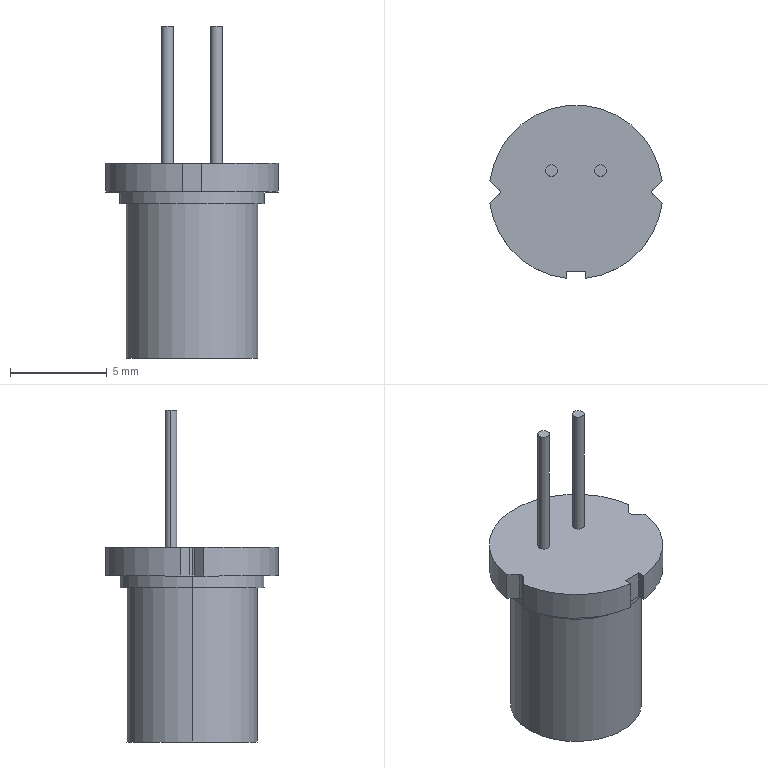Part | SolidWorks | features ICE 5, Dome 1, Extrusion 1, Fillet 1, MoveFace 1 | 1 solid | 31 faces | box 8.917 x 8.972 x 17.2 mm | volume 386.528 mm3 | cylinder 16 | plane 13 | sphere 2 | commonest cylinder face diameters 0.6 x4 0.4 x3 9 x3 5.8 x2 6.8 x2 7.5 x2
STEP:
#1=CARTESIAN_POINT('',(0.,0.,0.1));
#2=VERTEX_POINT('',#1);
#3=CARTESIAN_POINT('',(2.9,0.,3.));
#4=VERTEX_POINT('',#3);
#5=CARTESIAN_POINT('',(0.,0.,3.));
#6=DIRECTION('',(0.,-1.,0.));
#7=DIRECTION('',(1.,0.,0.));
#8=AXIS2_PLACEMENT_3D('',#5,#6,#7);
#9=CIRCLE('',#8,2.9);
#10=EDGE_CURVE('',#2,#4,#9,.T.);
#11=ORIENTED_EDGE('',*,*,#10,.F.);
#12=CARTESIAN_POINT('',(-2.9,0.,3.));
#13=VERTEX_POINT('',#12);
#14=CARTESIAN_POINT('',(0.,0.,3.));
#15=DIRECTION('',(0.,1.,0.));
#16=DIRECTION('',(-1.,0.,0.));
#17=AXIS2_PLACEMENT_3D('',#14,#15,#16);
#18=CIRCLE('',#17,2.9);
#19=EDGE_CURVE('',#2,#13,#18,.T.);
#20=ORIENTED_EDGE('',*,*,#19,.T.);
#21=CARTESIAN_POINT('',(0.,0.,3.));
#22=DIRECTION('',(0.,0.,-1.));
#23=DIRECTION('',(-1.,0.,0.));
#24=AXIS2_PLACEMENT_3D('',#21,#22,#23);
#25=CIRCLE('',#24,2.9);
#26=EDGE_CURVE('',#13,#4,#25,.T.);
#27=ORIENTED_EDGE('',*,*,#26,.T.);
#28=EDGE_LOOP('',(#11,#20,#27));
#29=FACE_OUTER_BOUND('',#28,.T.);
#30=CARTESIAN_POINT('',(0.,0.,3.));
#31=DIRECTION('',(0.,1.,0.));
#32=DIRECTION('',(1.,0.,0.));
#33=AXIS2_PLACEMENT_3D('',#30,#31,#32);
#34=SPHERICAL_SURFACE('',#33,2.9);
#35=ADVANCED_FACE('',(#29),#34,.T.);
#36=CARTESIAN_POINT('',(0.,0.,3.));
#37=DIRECTION('',(0.,0.,-1.));
#38=DIRECTION('',(-1.,0.,0.));
#39=AXIS2_PLACEMENT_3D('',#36,#37,#38);
#40=CIRCLE('',#39,2.9);
#41=EDGE_CURVE('',#4,#13,#40,.T.);
#42=ORIENTED_EDGE('',*,*,#41,.F.);
#43=CARTESIAN_POINT('',(2.9,0.,0.));
#44=VERTEX_POINT('',#43);
#45=CARTESIAN_POINT('',(2.9,0.,3.));
#46=DIRECTION('',(0.,0.,-1.));
#47=VECTOR('',#46,1000.);
#48=LINE('',#45,#47);
#49=EDGE_CURVE('',#4,#44,#48,.T.);
#50=ORIENTED_EDGE('',*,*,#49,.T.);
#51=CARTESIAN_POINT('',(-2.9,0.,0.));
#52=VERTEX_POINT('',#51);
#53=CARTESIAN_POINT('',(0.,0.,0.));
#54=DIRECTION('',(0.,0.,-1.));
#55=DIRECTION('',(-1.,0.,0.));
#56=AXIS2_PLACEMENT_3D('',#53,#54,#55);
#57=CIRCLE('',#56,2.9);
#58=EDGE_CURVE('',#44,#52,#57,.T.);
#59=ORIENTED_EDGE('',*,*,#58,.T.);
#60=CARTESIAN_POINT('',(-2.9,0.,3.));
#61=DIRECTION('',(0.,0.,-1.));
#62=VECTOR('',#61,1000.);
#63=LINE('',#60,#62);
#64=EDGE_CURVE('',#13,#52,#63,.T.);
#65=ORIENTED_EDGE('',*,*,#64,.F.);
#66=EDGE_LOOP('',(#42,#50,#59,#65));
#67=FACE_OUTER_BOUND('',#66,.T.);
#68=CARTESIAN_POINT('',(0.,0.,3.));
#69=DIRECTION('',(0.,0.,-1.));
#70=DIRECTION('',(-1.,0.,0.));
#71=AXIS2_PLACEMENT_3D('',#68,#69,#70);
#72=CYLINDRICAL_SURFACE('',#71,2.9);
#73=ADVANCED_FACE('',(#67),#72,.F.);
#74=CARTESIAN_POINT('',(3.4,0.,8.));
#75=VERTEX_POINT('',#74);
#76=CARTESIAN_POINT('',(-3.4,0.,8.));
#77=VERTEX_POINT('',#76);
#78=CARTESIAN_POINT('',(0.,0.,8.));
#79=DIRECTION('',(0.,0.,1.));
#80=DIRECTION('',(1.,0.,0.));
#81=AXIS2_PLACEMENT_3D('',#78,#79,#80);
#82=CIRCLE('',#81,3.4);
#83=EDGE_CURVE('',#75,#77,#82,.T.);
#84=ORIENTED_EDGE('',*,*,#83,.F.);
#85=CARTESIAN_POINT('',(3.4,0.,0.));
#86=VERTEX_POINT('',#85);
#87=CARTESIAN_POINT('',(3.4,0.,8.6));
#88=DIRECTION('',(0.,0.,-1.));
#89=VECTOR('',#88,1000.);
#90=LINE('',#87,#89);
#91=EDGE_CURVE('',#75,#86,#90,.T.);
#92=ORIENTED_EDGE('',*,*,#91,.T.);
#93=CARTESIAN_POINT('',(-3.4,0.,0.));
#94=VERTEX_POINT('',#93);
#95=CARTESIAN_POINT('',(0.,0.,0.));
#96=DIRECTION('',(0.,0.,1.));
#97=DIRECTION('',(1.,0.,0.));
#98=AXIS2_PLACEMENT_3D('',#95,#96,#97);
#99=CIRCLE('',#98,3.4);
#100=EDGE_CURVE('',#86,#94,#99,.T.);
#101=ORIENTED_EDGE('',*,*,#100,.T.);
#102=CARTESIAN_POINT('',(-3.4,0.,8.6));
#103=DIRECTION('',(0.,0.,-1.));
#104=VECTOR('',#103,1000.);
#105=LINE('',#102,#104);
#106=EDGE_CURVE('',#77,#94,#105,.T.);
#107=ORIENTED_EDGE('',*,*,#106,.F.);
#108=EDGE_LOOP('',(#84,#92,#101,#107));
#109=FACE_OUTER_BOUND('',#108,.T.);
#110=CARTESIAN_POINT('',(0.,0.,8.6));
#111=DIRECTION('',(0.,0.,-1.));
#112=DIRECTION('',(-1.,0.,0.));
#113=AXIS2_PLACEMENT_3D('',#110,#111,#112);
#114=CYLINDRICAL_SURFACE('',#113,3.4);
#115=ADVANCED_FACE('',(#109),#114,.T.);
#116=CARTESIAN_POINT('',(3.75,0.,8.));
#117=VERTEX_POINT('',#116);
#118=CARTESIAN_POINT('',(-3.75,0.,8.));
#119=VERTEX_POINT('',#118);
#120=CARTESIAN_POINT('',(0.,0.,8.));
#121=DIRECTION('',(0.,0.,1.));
#122=DIRECTION('',(1.,0.,0.));
#123=AXIS2_PLACEMENT_3D('',#120,#121,#122);
#124=CIRCLE('',#123,3.75);
#125=EDGE_CURVE('',#117,#119,#124,.T.);
#126=ORIENTED_EDGE('',*,*,#125,.T.);
#127=CARTESIAN_POINT('',(-3.75,0.,8.6));
#128=VERTEX_POINT('',#127);
#129=CARTESIAN_POINT('',(-3.75,0.,-4.807));
#130=DIRECTION('',(0.,0.,1.));
#131=VECTOR('',#130,1000.);
#132=LINE('',#129,#131);
#133=EDGE_CURVE('',#119,#128,#132,.T.);
#134=ORIENTED_EDGE('',*,*,#133,.T.);
#135=CARTESIAN_POINT('',(3.75,0.,8.6));
#136=VERTEX_POINT('',#135);
#137=CARTESIAN_POINT('',(0.,0.,8.6));
#138=DIRECTION('',(0.,0.,-1.));
#139=DIRECTION('',(1.,0.,0.));
#140=AXIS2_PLACEMENT_3D('',#137,#138,#139);
#141=CIRCLE('',#140,3.75);
#142=EDGE_CURVE('',#128,#136,#141,.T.);
#143=ORIENTED_EDGE('',*,*,#142,.T.);
#144=CARTESIAN_POINT('',(3.75,0.,-4.807));
#145=DIRECTION('',(0.,0.,1.));
#146=VECTOR('',#145,1000.);
#147=LINE('',#144,#146);
#148=EDGE_CURVE('',#117,#136,#147,.T.);
#149=ORIENTED_EDGE('',*,*,#148,.F.);
#150=EDGE_LOOP('',(#126,#134,#143,#149));
#151=FACE_OUTER_BOUND('',#150,.T.);
#152=CARTESIAN_POINT('',(0.,0.,-4.807));
#153=DIRECTION('',(0.,0.,1.));
#154=DIRECTION('',(1.,0.,0.));
#155=AXIS2_PLACEMENT_3D('',#152,#153,#154);
#156=CYLINDRICAL_SURFACE('',#155,3.75);
#157=ADVANCED_FACE('',(#151),#156,.T.);
#158=CARTESIAN_POINT('',(-3.933,0.,8.6));
#159=VERTEX_POINT('',#158);
#160=CARTESIAN_POINT('',(-3.991,0.1414,8.6));
#161=VERTEX_POINT('',#160);
#162=CARTESIAN_POINT('',(-4.133,0.,8.6));
#163=DIRECTION('',(0.,0.,1.));
#164=DIRECTION('',(1.,0.,0.));
#165=AXIS2_PLACEMENT_3D('',#162,#163,#164);
#166=CIRCLE('',#165,0.2);
#167=EDGE_CURVE('',#159,#161,#166,.T.);
#168=ORIENTED_EDGE('',*,*,#167,.F.);
#169=CARTESIAN_POINT('',(-3.933,0.,10.1));
#170=VERTEX_POINT('',#169);
#171=CARTESIAN_POINT('',(-3.933,0.,11.949));
#172=DIRECTION('',(0.,0.,1.));
#173=VECTOR('',#172,1000.);
#174=LINE('',#171,#173);
#175=EDGE_CURVE('',#159,#170,#174,.T.);
#176=ORIENTED_EDGE('',*,*,#175,.T.);
#177=CARTESIAN_POINT('',(-3.991,0.1414,10.1));
#178=VERTEX_POINT('',#177);
#179=CARTESIAN_POINT('',(-4.133,0.,10.1));
#180=DIRECTION('',(0.,0.,-1.));
#181=DIRECTION('',(1.,0.,0.));
#182=AXIS2_PLACEMENT_3D('',#179,#180,#181);
#183=CIRCLE('',#182,0.2);
#184=EDGE_CURVE('',#178,#170,#183,.T.);
#185=ORIENTED_EDGE('',*,*,#184,.F.);
#186=CARTESIAN_POINT('',(-3.991,0.1414,10.2));
#187=DIRECTION('',(0.,0.,1.));
#188=VECTOR('',#187,1000.);
#189=LINE('',#186,#188);
#190=EDGE_CURVE('',#161,#178,#189,.T.);
#191=ORIENTED_EDGE('',*,*,#190,.F.);
#192=EDGE_LOOP('',(#168,#176,#185,#191));
#193=FACE_OUTER_BOUND('',#192,.T.);
#194=CARTESIAN_POINT('',(-4.133,0.,11.949));
#195=DIRECTION('',(0.,0.,1.));
#196=DIRECTION('',(1.,0.,0.));
#197=AXIS2_PLACEMENT_3D('',#194,#195,#196);
#198=CYLINDRICAL_SURFACE('',#197,0.2);
#199=ADVANCED_FACE('',(#193),#198,.F.);
#200=CARTESIAN_POINT('',(1.57,1.1,17.2));
#201=VERTEX_POINT('',#200);
#202=CARTESIAN_POINT('',(0.97,1.1,17.2));
#203=VERTEX_POINT('',#202);
#204=CARTESIAN_POINT('',(1.27,1.1,17.2));
#205=DIRECTION('',(0.,0.,1.));
#206=DIRECTION('',(1.,0.,0.));
#207=AXIS2_PLACEMENT_3D('',#204,#205,#206);
#208=CIRCLE('',#207,0.3);
#209=EDGE_CURVE('',#201,#203,#208,.T.);
#210=ORIENTED_EDGE('',*,*,#209,.F.);
#211=CARTESIAN_POINT('',(1.57,1.1,10.1));
#212=VERTEX_POINT('',#211);
#213=CARTESIAN_POINT('',(1.57,1.1,17.2));
#214=DIRECTION('',(0.,0.,-1.));
#215=VECTOR('',#214,1000.);
#216=LINE('',#213,#215);
#217=EDGE_CURVE('',#201,#212,#216,.T.);
#218=ORIENTED_EDGE('',*,*,#217,.T.);
#219=CARTESIAN_POINT('',(0.97,1.1,10.1));
#220=VERTEX_POINT('',#219);
#221=CARTESIAN_POINT('',(1.27,1.1,10.1));
#222=DIRECTION('',(0.,0.,1.));
#223=DIRECTION('',(1.,0.,0.));
#224=AXIS2_PLACEMENT_3D('',#221,#222,#223);
#225=CIRCLE('',#224,0.3);
#226=EDGE_CURVE('',#212,#220,#225,.T.);
#227=ORIENTED_EDGE('',*,*,#226,.T.);
#228=CARTESIAN_POINT('',(0.97,1.1,17.2));
#229=DIRECTION('',(0.,0.,-1.));
#230=VECTOR('',#229,1000.);
#231=LINE('',#228,#230);
#232=EDGE_CURVE('',#203,#220,#231,.T.);
#233=ORIENTED_EDGE('',*,*,#232,.F.);
#234=EDGE_LOOP('',(#210,#218,#227,#233));
#235=FACE_OUTER_BOUND('',#234,.T.);
#236=CARTESIAN_POINT('',(1.27,1.1,17.2));
#237=DIRECTION('',(0.,0.,-1.));
#238=DIRECTION('',(-1.,0.,0.));
#239=AXIS2_PLACEMENT_3D('',#236,#237,#238);
#240=CYLINDRICAL_SURFACE('',#239,0.3);
#241=ADVANCED_FACE('',(#235),#240,.T.);
#242=CARTESIAN_POINT('',(-0.97,1.1,17.2));
#243=VERTEX_POINT('',#242);
#244=CARTESIAN_POINT('',(-1.57,1.1,17.2));
#245=VERTEX_POINT('',#244);
#246=CARTESIAN_POINT('',(-1.27,1.1,17.2));
#247=DIRECTION('',(0.,0.,1.));
#248=DIRECTION('',(1.,0.,0.));
#249=AXIS2_PLACEMENT_3D('',#246,#247,#248);
#250=CIRCLE('',#249,0.3);
#251=EDGE_CURVE('',#243,#245,#250,.T.);
#252=ORIENTED_EDGE('',*,*,#251,.F.);
#253=CARTESIAN_POINT('',(-0.97,1.1,10.1));
#254=VERTEX_POINT('',#253);
#255=CARTESIAN_POINT('',(-0.97,1.1,17.2));
#256=DIRECTION('',(0.,0.,-1.));
#257=VECTOR('',#256,1000.);
#258=LINE('',#255,#257);
#259=EDGE_CURVE('',#243,#254,#258,.T.);
#260=ORIENTED_EDGE('',*,*,#259,.T.);
#261=CARTESIAN_POINT('',(-1.57,1.1,10.1));
#262=VERTEX_POINT('',#261);
#263=CARTESIAN_POINT('',(-1.27,1.1,10.1));
#264=DIRECTION('',(0.,0.,1.));
#265=DIRECTION('',(1.,0.,0.));
#266=AXIS2_PLACEMENT_3D('',#263,#264,#265);
#267=CIRCLE('',#266,0.3);
#268=EDGE_CURVE('',#254,#262,#267,.T.);
#269=ORIENTED_EDGE('',*,*,#268,.T.);
#270=CARTESIAN_POINT('',(-1.57,1.1,17.2));
#271=DIRECTION('',(0.,0.,-1.));
#272=VECTOR('',#271,1000.);
#273=LINE('',#270,#272);
#274=EDGE_CURVE('',#245,#262,#273,.T.);
#275=ORIENTED_EDGE('',*,*,#274,.F.);
#276=EDGE_LOOP('',(#252,#260,#269,#275));
#277=FACE_OUTER_BOUND('',#276,.T.);
#278=CARTESIAN_POINT('',(-1.27,1.1,17.2));
#279=DIRECTION('',(0.,0.,-1.));
#280=DIRECTION('',(-1.,0.,0.));
#281=AXIS2_PLACEMENT_3D('',#278,#279,#280);
#282=CYLINDRICAL_SURFACE('',#281,0.3);
#283=ADVANCED_FACE('',(#277),#282,.T.);
#284=CARTESIAN_POINT('',(-4.459,-0.6086,8.6));
#285=VERTEX_POINT('',#284);
#286=CARTESIAN_POINT('',(-0.5,-4.472,8.6));
#287=VERTEX_POINT('',#286);
#288=CARTESIAN_POINT('',(0.,0.,8.6));
#289=DIRECTION('',(0.,0.,1.));
#290=DIRECTION('',(1.,0.,0.));
#291=AXIS2_PLACEMENT_3D('',#288,#289,#290);
#292=CIRCLE('',#291,4.5);
#293=EDGE_CURVE('',#285,#287,#292,.T.);
#294=ORIENTED_EDGE('',*,*,#293,.T.);
#295=CARTESIAN_POINT('',(-0.5,-4.472,10.1));
#296=VERTEX_POINT('',#295);
#297=CARTESIAN_POINT('',(-0.5,-4.472,10.2));
#298=DIRECTION('',(0.,0.,1.));
#299=VECTOR('',#298,1000.);
#300=LINE('',#297,#299);
#301=EDGE_CURVE('',#287,#296,#300,.T.);
#302=ORIENTED_EDGE('',*,*,#301,.T.);
#303=CARTESIAN_POINT('',(-4.459,-0.6086,10.1));
#304=VERTEX_POINT('',#303);
#305=CARTESIAN_POINT('',(0.,0.,10.1));
#306=DIRECTION('',(0.,0.,1.));
#307=DIRECTION('',(1.,0.,0.));
#308=AXIS2_PLACEMENT_3D('',#305,#306,#307);
#309=CIRCLE('',#308,4.5);
#310=EDGE_CURVE('',#304,#296,#309,.T.);
#311=ORIENTED_EDGE('',*,*,#310,.F.);
#312=CARTESIAN_POINT('',(-4.459,-0.6086,10.2));
#313=DIRECTION('',(0.,0.,-1.));
#314=VECTOR('',#313,1000.);
#315=LINE('',#312,#314);
#316=EDGE_CURVE('',#304,#285,#315,.T.);
#317=ORIENTED_EDGE('',*,*,#316,.T.);
#318=EDGE_LOOP('',(#294,#302,#311,#317));
#319=FACE_OUTER_BOUND('',#318,.T.);
#320=CARTESIAN_POINT('',(0.,0.,10.2));
#321=DIRECTION('',(0.,0.,-1.));
#322=DIRECTION('',(-1.,0.,0.));
#323=AXIS2_PLACEMENT_3D('',#320,#321,#322);
#324=CYLINDRICAL_SURFACE('',#323,4.5);
#325=ADVANCED_FACE('',(#319),#324,.T.);
#326=CARTESIAN_POINT('',(4.459,0.6086,8.6));
#327=VERTEX_POINT('',#326);
#328=CARTESIAN_POINT('',(-4.459,0.6086,8.6));
#329=VERTEX_POINT('',#328);
#330=CARTESIAN_POINT('',(0.,0.,8.6));
#331=DIRECTION('',(0.,0.,1.));
#332=DIRECTION('',(1.,0.,0.));
#333=AXIS2_PLACEMENT_3D('',#330,#331,#332);
#334=CIRCLE('',#333,4.5);
#335=EDGE_CURVE('',#327,#329,#334,.T.);
#336=ORIENTED_EDGE('',*,*,#335,.T.);
#337=CARTESIAN_POINT('',(-4.459,0.6086,10.1));
#338=VERTEX_POINT('',#337);
#339=CARTESIAN_POINT('',(-4.459,0.6086,10.2));
#340=DIRECTION('',(0.,0.,1.));
#341=VECTOR('',#340,1000.);
#342=LINE('',#339,#341);
#343=EDGE_CURVE('',#329,#338,#342,.T.);
#344=ORIENTED_EDGE('',*,*,#343,.T.);
#345=CARTESIAN_POINT('',(4.459,0.6086,10.1));
#346=VERTEX_POINT('',#345);
#347=CARTESIAN_POINT('',(0.,0.,10.1));
#348=DIRECTION('',(0.,0.,1.));
#349=DIRECTION('',(1.,0.,0.));
#350=AXIS2_PLACEMENT_3D('',#347,#348,#349);
#351=CIRCLE('',#350,4.5);
#352=EDGE_CURVE('',#346,#338,#351,.T.);
#353=ORIENTED_EDGE('',*,*,#352,.F.);
#354=CARTESIAN_POINT('',(4.459,0.6086,10.2));
#355=DIRECTION('',(0.,0.,-1.));
#356=VECTOR('',#355,1000.);
#357=LINE('',#354,#356);
#358=EDGE_CURVE('',#346,#327,#357,.T.);
#359=ORIENTED_EDGE('',*,*,#358,.T.);
#360=EDGE_LOOP('',(#336,#344,#353,#359));
#361=FACE_OUTER_BOUND('',#360,.T.);
#362=CARTESIAN_POINT('',(0.,0.,10.2));
#363=DIRECTION('',(0.,0.,-1.));
#364=DIRECTION('',(-1.,0.,0.));
#365=AXIS2_PLACEMENT_3D('',#362,#363,#364);
#366=CYLINDRICAL_SURFACE('',#365,4.5);
#367=ADVANCED_FACE('',(#361),#366,.T.);
#368=CARTESIAN_POINT('',(0.5,-4.472,10.1));
#369=VERTEX_POINT('',#368);
#370=CARTESIAN_POINT('',(4.459,-0.6086,10.1));
#371=VERTEX_POINT('',#370);
#372=CARTESIAN_POINT('',(0.,0.,10.1));
#373=DIRECTION('',(0.,0.,1.));
#374=DIRECTION('',(1.,0.,0.));
#375=AXIS2_PLACEMENT_3D('',#372,#373,#374);
#376=CIRCLE('',#375,4.5);
#377=EDGE_CURVE('',#369,#371,#376,.T.);
#378=ORIENTED_EDGE('',*,*,#377,.F.);
#379=CARTESIAN_POINT('',(0.5,-4.472,8.6));
#380=VERTEX_POINT('',#379);
#381=CARTESIAN_POINT('',(0.5,-4.472,10.2));
#382=DIRECTION('',(0.,0.,-1.));
#383=VECTOR('',#382,1000.);
#384=LINE('',#381,#383);
#385=EDGE_CURVE('',#369,#380,#384,.T.);
#386=ORIENTED_EDGE('',*,*,#385,.T.);
#387=CARTESIAN_POINT('',(4.459,-0.6086,8.6));
#388=VERTEX_POINT('',#387);
#389=CARTESIAN_POINT('',(0.,0.,8.6));
#390=DIRECTION('',(0.,0.,1.));
#391=DIRECTION('',(1.,0.,0.));
#392=AXIS2_PLACEMENT_3D('',#389,#390,#391);
#393=CIRCLE('',#392,4.5);
#394=EDGE_CURVE('',#380,#388,#393,.T.);
#395=ORIENTED_EDGE('',*,*,#394,.T.);
#396=CARTESIAN_POINT('',(4.459,-0.6086,10.2));
#397=DIRECTION('',(0.,0.,1.));
#398=VECTOR('',#397,1000.);
#399=LINE('',#396,#398);
#400=EDGE_CURVE('',#388,#371,#399,.T.);
#401=ORIENTED_EDGE('',*,*,#400,.T.);
#402=EDGE_LOOP('',(#378,#386,#395,#401));
#403=FACE_OUTER_BOUND('',#402,.T.);
#404=CARTESIAN_POINT('',(0.,0.,10.2));
#405=DIRECTION('',(0.,0.,-1.));
#406=DIRECTION('',(-1.,0.,0.));
#407=AXIS2_PLACEMENT_3D('',#404,#405,#406);
#408=CYLINDRICAL_SURFACE('',#407,4.5);
#409=ADVANCED_FACE('',(#403),#408,.T.);
#410=CARTESIAN_POINT('',(-0.5,-4.1,10.1));
#411=VERTEX_POINT('',#410);
#412=CARTESIAN_POINT('',(-0.5,-4.735,10.1));
#413=DIRECTION('',(0.,1.,0.));
#414=VECTOR('',#413,1000.);
#415=LINE('',#412,#414);
#416=EDGE_CURVE('',#296,#411,#415,.T.);
#417=ORIENTED_EDGE('',*,*,#416,.T.);
#418=CARTESIAN_POINT('',(0.5,-4.1,10.1));
#419=VERTEX_POINT('',#418);
#420=CARTESIAN_POINT('',(0.5,-4.1,10.1));
#421=DIRECTION('',(1.,0.,0.));
#422=VECTOR('',#421,1000.);
#423=LINE('',#420,#422);
#424=EDGE_CURVE('',#411,#419,#423,.T.);
#425=ORIENTED_EDGE('',*,*,#424,.T.);
#426=CARTESIAN_POINT('',(0.5,-4.735,10.1));
#427=DIRECTION('',(0.,-1.,0.));
#428=VECTOR('',#427,1000.);
#429=LINE('',#426,#428);
#430=EDGE_CURVE('',#419,#369,#429,.T.);
#431=ORIENTED_EDGE('',*,*,#430,.T.);
#432=ORIENTED_EDGE('',*,*,#377,.T.);
#433=CARTESIAN_POINT('',(3.991,-0.1414,10.1));
#434=VERTEX_POINT('',#433);
#435=CARTESIAN_POINT('',(3.85,0.,10.1));
#436=DIRECTION('',(-0.7071,0.7071,0.));
#437=VECTOR('',#436,1000.);
#438=LINE('',#435,#437);
#439=EDGE_CURVE('',#371,#434,#438,.T.);
#440=ORIENTED_EDGE('',*,*,#439,.T.);
#441=CARTESIAN_POINT('',(3.991,0.1414,10.1));
#442=VERTEX_POINT('',#441);
#443=CARTESIAN_POINT('',(4.133,0.,10.1));
#444=DIRECTION('',(0.,0.,-1.));
#445=DIRECTION('',(1.,0.,0.));
#446=AXIS2_PLACEMENT_3D('',#443,#444,#445);
#447=CIRCLE('',#446,0.2);
#448=EDGE_CURVE('',#434,#442,#447,.T.);
#449=ORIENTED_EDGE('',*,*,#448,.T.);
#450=CARTESIAN_POINT('',(4.633,0.7827,10.1));
#451=DIRECTION('',(0.7071,0.7071,0.));
#452=VECTOR('',#451,1000.);
#453=LINE('',#450,#452);
#454=EDGE_CURVE('',#442,#346,#453,.T.);
#455=ORIENTED_EDGE('',*,*,#454,.T.);
#456=ORIENTED_EDGE('',*,*,#352,.T.);
#457=CARTESIAN_POINT('',(-4.633,0.7827,10.1));
#458=DIRECTION('',(0.7071,-0.7071,0.));
#459=VECTOR('',#458,1000.);
#460=LINE('',#457,#459);
#461=EDGE_CURVE('',#338,#178,#460,.T.);
#462=ORIENTED_EDGE('',*,*,#461,.T.);
#463=ORIENTED_EDGE('',*,*,#184,.T.);
#464=CARTESIAN_POINT('',(-3.991,-0.1414,10.1));
#465=VERTEX_POINT('',#464);
#466=CARTESIAN_POINT('',(-4.133,0.,10.1));
#467=DIRECTION('',(0.,0.,-1.));
#468=DIRECTION('',(1.,0.,0.));
#469=AXIS2_PLACEMENT_3D('',#466,#467,#468);
#470=CIRCLE('',#469,0.2);
#471=EDGE_CURVE('',#170,#465,#470,.T.);
#472=ORIENTED_EDGE('',*,*,#471,.T.);
#473=CARTESIAN_POINT('',(-3.85,0.,10.1));
#474=DIRECTION('',(-0.7071,-0.7071,0.));
#475=VECTOR('',#474,1000.);
#476=LINE('',#473,#475);
#477=EDGE_CURVE('',#465,#304,#476,.T.);
#478=ORIENTED_EDGE('',*,*,#477,.T.);
#479=ORIENTED_EDGE('',*,*,#310,.T.);
#480=EDGE_LOOP('',(#417,#425,#431,#432,#440,#449,#455,#456,#462,#463,#472,#478,#479));
#481=FACE_OUTER_BOUND('',#480,.T.);
#482=CARTESIAN_POINT('',(1.27,1.1,10.1));
#483=DIRECTION('',(0.,0.,1.));
#484=DIRECTION('',(1.,0.,0.));
#485=AXIS2_PLACEMENT_3D('',#482,#483,#484);
#486=CIRCLE('',#485,0.3);
#487=EDGE_CURVE('',#220,#212,#486,.T.);
#488=ORIENTED_EDGE('',*,*,#487,.F.);
#489=ORIENTED_EDGE('',*,*,#226,.F.);
#490=EDGE_LOOP('',(#488,#489));
#491=FACE_BOUND('',#490,.T.);
#492=CARTESIAN_POINT('',(-1.27,1.1,10.1));
#493=DIRECTION('',(0.,0.,1.));
#494=DIRECTION('',(1.,0.,0.));
#495=AXIS2_PLACEMENT_3D('',#492,#493,#494);
#496=CIRCLE('',#495,0.3);
#497=EDGE_CURVE('',#262,#254,#496,.T.);
#498=ORIENTED_EDGE('',*,*,#497,.F.);
#499=ORIENTED_EDGE('',*,*,#268,.F.);
#500=EDGE_LOOP('',(#498,#499));
#501=FACE_BOUND('',#500,.T.);
#502=CARTESIAN_POINT('',(0.,0.,10.1));
#503=DIRECTION('',(0.,0.,1.));
#504=DIRECTION('',(1.,0.,0.));
#505=AXIS2_PLACEMENT_3D('',#502,#503,#504);
#506=PLANE('',#505);
#507=ADVANCED_FACE('',(#481,#491,#501),#506,.T.);
#508=CARTESIAN_POINT('',(0.,0.,8.6));
#509=DIRECTION('',(0.,0.,-1.));
#510=DIRECTION('',(1.,0.,0.));
#511=AXIS2_PLACEMENT_3D('',#508,#509,#510);
#512=CIRCLE('',#511,3.75);
#513=EDGE_CURVE('',#136,#128,#512,.T.);
#514=ORIENTED_EDGE('',*,*,#513,.F.);
#515=ORIENTED_EDGE('',*,*,#142,.F.);
#516=EDGE_LOOP('',(#514,#515));
#517=FACE_BOUND('',#516,.T.);
#518=CARTESIAN_POINT('',(-0.5,-4.1,8.6));
#519=VERTEX_POINT('',#518);
#520=CARTESIAN_POINT('',(0.5,-4.1,8.6));
#521=VERTEX_POINT('',#520);
#522=CARTESIAN_POINT('',(0.5,-4.1,8.6));
#523=DIRECTION('',(1.,0.,0.));
#524=VECTOR('',#523,1000.);
#525=LINE('',#522,#524);
#526=EDGE_CURVE('',#519,#521,#525,.T.);
#527=ORIENTED_EDGE('',*,*,#526,.F.);
#528=CARTESIAN_POINT('',(-0.5,0.,8.6));
#529=DIRECTION('',(0.,-1.,0.));
#530=VECTOR('',#529,1000.);
#531=LINE('',#528,#530);
#532=EDGE_CURVE('',#519,#287,#531,.T.);
#533=ORIENTED_EDGE('',*,*,#532,.T.);
#534=ORIENTED_EDGE('',*,*,#293,.F.);
#535=CARTESIAN_POINT('',(-3.991,-0.1414,8.6));
#536=VERTEX_POINT('',#535);
#537=CARTESIAN_POINT('',(-3.85,0.,8.6));
#538=DIRECTION('',(-0.7071,-0.7071,0.));
#539=VECTOR('',#538,1000.);
#540=LINE('',#537,#539);
#541=EDGE_CURVE('',#536,#285,#540,.T.);
#542=ORIENTED_EDGE('',*,*,#541,.F.);
#543=CARTESIAN_POINT('',(-4.133,0.,8.6));
#544=DIRECTION('',(0.,0.,1.));
#545=DIRECTION('',(1.,0.,0.));
#546=AXIS2_PLACEMENT_3D('',#543,#544,#545);
#547=CIRCLE('',#546,0.2);
#548=EDGE_CURVE('',#536,#159,#547,.T.);
#549=ORIENTED_EDGE('',*,*,#548,.T.);
#550=ORIENTED_EDGE('',*,*,#167,.T.);
#551=CARTESIAN_POINT('',(-1.925,-1.925,8.6));
#552=DIRECTION('',(-0.7071,0.7071,0.));
#553=VECTOR('',#552,1000.);
#554=LINE('',#551,#553);
#555=EDGE_CURVE('',#161,#329,#554,.T.);
#556=ORIENTED_EDGE('',*,*,#555,.T.);
#557=ORIENTED_EDGE('',*,*,#335,.F.);
#558=CARTESIAN_POINT('',(3.991,0.1414,8.6));
#559=VERTEX_POINT('',#558);
#560=CARTESIAN_POINT('',(4.633,0.7827,8.6));
#561=DIRECTION('',(0.7071,0.7071,0.));
#562=VECTOR('',#561,1000.);
#563=LINE('',#560,#562);
#564=EDGE_CURVE('',#559,#327,#563,.T.);
#565=ORIENTED_EDGE('',*,*,#564,.F.);
#566=CARTESIAN_POINT('',(3.991,-0.1414,8.6));
#567=VERTEX_POINT('',#566);
#568=CARTESIAN_POINT('',(4.133,0.,8.6));
#569=DIRECTION('',(0.,0.,1.));
#570=DIRECTION('',(1.,0.,0.));
#571=AXIS2_PLACEMENT_3D('',#568,#569,#570);
#572=CIRCLE('',#571,0.2);
#573=EDGE_CURVE('',#559,#567,#572,.T.);
#574=ORIENTED_EDGE('',*,*,#573,.T.);
#575=CARTESIAN_POINT('',(1.925,1.925,8.6));
#576=DIRECTION('',(0.7071,-0.7071,0.));
#577=VECTOR('',#576,1000.);
#578=LINE('',#575,#577);
#579=EDGE_CURVE('',#567,#388,#578,.T.);
#580=ORIENTED_EDGE('',*,*,#579,.T.);
#581=ORIENTED_EDGE('',*,*,#394,.F.);
#582=CARTESIAN_POINT('',(0.5,-4.735,8.6));
#583=DIRECTION('',(0.,-1.,0.));
#584=VECTOR('',#583,1000.);
#585=LINE('',#582,#584);
#586=EDGE_CURVE('',#521,#380,#585,.T.);
#587=ORIENTED_EDGE('',*,*,#586,.F.);
#588=EDGE_LOOP('',(#527,#533,#534,#542,#549,#550,#556,#557,#565,#574,#580,#581,#587));
#589=FACE_OUTER_BOUND('',#588,.T.);
#590=CARTESIAN_POINT('',(0.,0.,8.6));
#591=DIRECTION('',(0.,0.,1.));
#592=DIRECTION('',(1.,0.,0.));
#593=AXIS2_PLACEMENT_3D('',#590,#591,#592);
#594=PLANE('',#593);
#595=ADVANCED_FACE('',(#517,#589),#594,.F.);
#596=ORIENTED_EDGE('',*,*,#259,.F.);
#597=CARTESIAN_POINT('',(-1.27,1.1,17.2));
#598=DIRECTION('',(0.,0.,1.));
#599=DIRECTION('',(1.,0.,0.));
#600=AXIS2_PLACEMENT_3D('',#597,#598,#599);
#601=CIRCLE('',#600,0.3);
#602=EDGE_CURVE('',#245,#243,#601,.T.);
#603=ORIENTED_EDGE('',*,*,#602,.F.);
#604=ORIENTED_EDGE('',*,*,#274,.T.);
#605=ORIENTED_EDGE('',*,*,#497,.T.);
#606=EDGE_LOOP('',(#596,#603,#604,#605));
#607=FACE_OUTER_BOUND('',#606,.T.);
#608=CARTESIAN_POINT('',(-1.27,1.1,17.2));
#609=DIRECTION('',(0.,0.,-1.));
#610=DIRECTION('',(-1.,0.,0.));
#611=AXIS2_PLACEMENT_3D('',#608,#609,#610);
#612=CYLINDRICAL_SURFACE('',#611,0.3);
#613=ADVANCED_FACE('',(#607),#612,.T.);
#614=ORIENTED_EDGE('',*,*,#602,.T.);
#615=ORIENTED_EDGE('',*,*,#251,.T.);
#616=EDGE_LOOP('',(#614,#615));
#617=FACE_OUTER_BOUND('',#616,.T.);
#618=CARTESIAN_POINT('',(-1.27,1.1,17.2));
#619=DIRECTION('',(0.,0.,1.));
#620=DIRECTION('',(1.,0.,0.));
#621=AXIS2_PLACEMENT_3D('',#618,#619,#620);
#622=PLANE('',#621);
#623=ADVANCED_FACE('',(#617),#622,.T.);
#624=ORIENTED_EDGE('',*,*,#217,.F.);
#625=CARTESIAN_POINT('',(1.27,1.1,17.2));
#626=DIRECTION('',(0.,0.,1.));
#627=DIRECTION('',(1.,0.,0.));
#628=AXIS2_PLACEMENT_3D('',#625,#626,#627);
#629=CIRCLE('',#628,0.3);
#630=EDGE_CURVE('',#203,#201,#629,.T.);
#631=ORIENTED_EDGE('',*,*,#630,.F.);
#632=ORIENTED_EDGE('',*,*,#232,.T.);
#633=ORIENTED_EDGE('',*,*,#487,.T.);
#634=EDGE_LOOP('',(#624,#631,#632,#633));
#635=FACE_OUTER_BOUND('',#634,.T.);
#636=CARTESIAN_POINT('',(1.27,1.1,17.2));
#637=DIRECTION('',(0.,0.,-1.));
#638=DIRECTION('',(-1.,0.,0.));
#639=AXIS2_PLACEMENT_3D('',#636,#637,#638);
#640=CYLINDRICAL_SURFACE('',#639,0.3);
#641=ADVANCED_FACE('',(#635),#640,.T.);
#642=ORIENTED_EDGE('',*,*,#630,.T.);
#643=ORIENTED_EDGE('',*,*,#209,.T.);
#644=EDGE_LOOP('',(#642,#643));
#645=FACE_OUTER_BOUND('',#644,.T.);
#646=CARTESIAN_POINT('',(1.27,1.1,17.2));
#647=DIRECTION('',(0.,0.,1.));
#648=DIRECTION('',(1.,0.,0.));
#649=AXIS2_PLACEMENT_3D('',#646,#647,#648);
#650=PLANE('',#649);
#651=ADVANCED_FACE('',(#645),#650,.T.);
#652=ORIENTED_EDGE('',*,*,#579,.F.);
#653=CARTESIAN_POINT('',(3.991,-0.1414,10.2));
#654=DIRECTION('',(0.,0.,1.));
#655=VECTOR('',#654,1000.);
#656=LINE('',#653,#655);
#657=EDGE_CURVE('',#567,#434,#656,.T.);
#658=ORIENTED_EDGE('',*,*,#657,.T.);
#659=ORIENTED_EDGE('',*,*,#439,.F.);
#660=ORIENTED_EDGE('',*,*,#400,.F.);
#661=EDGE_LOOP('',(#652,#658,#659,#660));
#662=FACE_OUTER_BOUND('',#661,.T.);
#663=CARTESIAN_POINT('',(3.85,0.,11.949));
#664=DIRECTION('',(-0.7071,-0.7071,0.));
#665=DIRECTION('',(0.7071,-0.7071,0.));
#666=AXIS2_PLACEMENT_3D('',#663,#664,#665);
#667=PLANE('',#666);
#668=ADVANCED_FACE('',(#662),#667,.F.);
#669=ORIENTED_EDGE('',*,*,#454,.F.);
#670=CARTESIAN_POINT('',(3.991,0.1414,8.6));
#671=DIRECTION('',(0.,0.,-1.));
#672=VECTOR('',#671,1000.);
#673=LINE('',#670,#672);
#674=EDGE_CURVE('',#442,#559,#673,.T.);
#675=ORIENTED_EDGE('',*,*,#674,.T.);
#676=ORIENTED_EDGE('',*,*,#564,.T.);
#677=ORIENTED_EDGE('',*,*,#358,.F.);
#678=EDGE_LOOP('',(#669,#675,#676,#677));
#679=FACE_OUTER_BOUND('',#678,.T.);
#680=CARTESIAN_POINT('',(4.633,0.7827,11.949));
#681=DIRECTION('',(-0.7071,0.7071,0.));
#682=DIRECTION('',(-0.7071,-0.7071,0.));
#683=AXIS2_PLACEMENT_3D('',#680,#681,#682);
#684=PLANE('',#683);
#685=ADVANCED_FACE('',(#679),#684,.F.);
#686=ORIENTED_EDGE('',*,*,#555,.F.);
#687=ORIENTED_EDGE('',*,*,#190,.T.);
#688=ORIENTED_EDGE('',*,*,#461,.F.);
#689=ORIENTED_EDGE('',*,*,#343,.F.);
#690=EDGE_LOOP('',(#686,#687,#688,#689));
#691=FACE_OUTER_BOUND('',#690,.T.);
#692=CARTESIAN_POINT('',(-4.633,0.7827,11.949));
#693=DIRECTION('',(0.7071,0.7071,0.));
#694=DIRECTION('',(-0.7071,0.7071,0.));
#695=AXIS2_PLACEMENT_3D('',#692,#693,#694);
#696=PLANE('',#695);
#697=ADVANCED_FACE('',(#691),#696,.F.);
#698=ORIENTED_EDGE('',*,*,#477,.F.);
#699=CARTESIAN_POINT('',(-3.991,-0.1414,8.6));
#700=DIRECTION('',(0.,0.,-1.));
#701=VECTOR('',#700,1000.);
#702=LINE('',#699,#701);
#703=EDGE_CURVE('',#465,#536,#702,.T.);
#704=ORIENTED_EDGE('',*,*,#703,.T.);
#705=ORIENTED_EDGE('',*,*,#541,.T.);
#706=ORIENTED_EDGE('',*,*,#316,.F.);
#707=EDGE_LOOP('',(#698,#704,#705,#706));
#708=FACE_OUTER_BOUND('',#707,.T.);
#709=CARTESIAN_POINT('',(-3.85,0.,11.949));
#710=DIRECTION('',(0.7071,-0.7071,0.));
#711=DIRECTION('',(0.7071,0.7071,0.));
#712=AXIS2_PLACEMENT_3D('',#709,#710,#711);
#713=PLANE('',#712);
#714=ADVANCED_FACE('',(#708),#713,.F.);
#715=ORIENTED_EDGE('',*,*,#532,.F.);
#716=CARTESIAN_POINT('',(-0.5,-4.1,11.949));
#717=DIRECTION('',(0.,0.,-1.));
#718=VECTOR('',#717,1000.);
#719=LINE('',#716,#718);
#720=EDGE_CURVE('',#411,#519,#719,.T.);
#721=ORIENTED_EDGE('',*,*,#720,.F.);
#722=ORIENTED_EDGE('',*,*,#416,.F.);
#723=ORIENTED_EDGE('',*,*,#301,.F.);
#724=EDGE_LOOP('',(#715,#721,#722,#723));
#725=FACE_OUTER_BOUND('',#724,.T.);
#726=CARTESIAN_POINT('',(-0.5,-4.735,11.949));
#727=DIRECTION('',(-1.,0.,0.));
#728=DIRECTION('',(0.,-1.,0.));
#729=AXIS2_PLACEMENT_3D('',#726,#727,#728);
#730=PLANE('',#729);
#731=ADVANCED_FACE('',(#725),#730,.F.);
#732=ORIENTED_EDGE('',*,*,#430,.F.);
#733=CARTESIAN_POINT('',(0.5,-4.1,11.949));
#734=DIRECTION('',(0.,0.,-1.));
#735=VECTOR('',#734,1000.);
#736=LINE('',#733,#735);
#737=EDGE_CURVE('',#419,#521,#736,.T.);
#738=ORIENTED_EDGE('',*,*,#737,.T.);
#739=ORIENTED_EDGE('',*,*,#586,.T.);
#740=ORIENTED_EDGE('',*,*,#385,.F.);
#741=EDGE_LOOP('',(#732,#738,#739,#740));
#742=FACE_OUTER_BOUND('',#741,.T.);
#743=CARTESIAN_POINT('',(0.5,-4.735,11.949));
#744=DIRECTION('',(1.,0.,0.));
#745=DIRECTION('',(0.,1.,0.));
#746=AXIS2_PLACEMENT_3D('',#743,#744,#745);
#747=PLANE('',#746);
#748=ADVANCED_FACE('',(#742),#747,.F.);
#749=ORIENTED_EDGE('',*,*,#720,.T.);
#750=ORIENTED_EDGE('',*,*,#526,.T.);
#751=ORIENTED_EDGE('',*,*,#737,.F.);
#752=ORIENTED_EDGE('',*,*,#424,.F.);
#753=EDGE_LOOP('',(#749,#750,#751,#752));
#754=FACE_OUTER_BOUND('',#753,.T.);
#755=CARTESIAN_POINT('',(0.5,-4.1,11.949));
#756=DIRECTION('',(0.,1.,0.));
#757=DIRECTION('',(0.,0.,1.));
#758=AXIS2_PLACEMENT_3D('',#755,#756,#757);
#759=PLANE('',#758);
#760=ADVANCED_FACE('',(#754),#759,.F.);
#761=ORIENTED_EDGE('',*,*,#175,.F.);
#762=ORIENTED_EDGE('',*,*,#548,.F.);
#763=ORIENTED_EDGE('',*,*,#703,.F.);
#764=ORIENTED_EDGE('',*,*,#471,.F.);
#765=EDGE_LOOP('',(#761,#762,#763,#764));
#766=FACE_OUTER_BOUND('',#765,.T.);
#767=CARTESIAN_POINT('',(-4.133,0.,11.949));
#768=DIRECTION('',(0.,0.,1.));
#769=DIRECTION('',(1.,0.,0.));
#770=AXIS2_PLACEMENT_3D('',#767,#768,#769);
#771=CYLINDRICAL_SURFACE('',#770,0.2);
#772=ADVANCED_FACE('',(#766),#771,.F.);
#773=ORIENTED_EDGE('',*,*,#448,.F.);
#774=ORIENTED_EDGE('',*,*,#657,.F.);
#775=ORIENTED_EDGE('',*,*,#573,.F.);
#776=ORIENTED_EDGE('',*,*,#674,.F.);
#777=EDGE_LOOP('',(#773,#774,#775,#776));
#778=FACE_OUTER_BOUND('',#777,.T.);
#779=CARTESIAN_POINT('',(4.133,0.,11.949));
#780=DIRECTION('',(0.,0.,1.));
#781=DIRECTION('',(1.,0.,0.));
#782=AXIS2_PLACEMENT_3D('',#779,#780,#781);
#783=CYLINDRICAL_SURFACE('',#782,0.2);
#784=ADVANCED_FACE('',(#778),#783,.F.);
#785=ORIENTED_EDGE('',*,*,#133,.F.);
#786=CARTESIAN_POINT('',(0.,0.,8.));
#787=DIRECTION('',(0.,0.,1.));
#788=DIRECTION('',(1.,0.,0.));
#789=AXIS2_PLACEMENT_3D('',#786,#787,#788);
#790=CIRCLE('',#789,3.75);
#791=EDGE_CURVE('',#119,#117,#790,.T.);
#792=ORIENTED_EDGE('',*,*,#791,.T.);
#793=ORIENTED_EDGE('',*,*,#148,.T.);
#794=ORIENTED_EDGE('',*,*,#513,.T.);
#795=EDGE_LOOP('',(#785,#792,#793,#794));
#796=FACE_OUTER_BOUND('',#795,.T.);
#797=CARTESIAN_POINT('',(0.,0.,-4.807));
#798=DIRECTION('',(0.,0.,1.));
#799=DIRECTION('',(1.,0.,0.));
#800=AXIS2_PLACEMENT_3D('',#797,#798,#799);
#801=CYLINDRICAL_SURFACE('',#800,3.75);
#802=ADVANCED_FACE('',(#796),#801,.T.);
#803=CARTESIAN_POINT('',(0.,0.,8.));
#804=DIRECTION('',(0.,0.,1.));
#805=DIRECTION('',(1.,0.,0.));
#806=AXIS2_PLACEMENT_3D('',#803,#804,#805);
#807=CIRCLE('',#806,3.4);
#808=EDGE_CURVE('',#77,#75,#807,.T.);
#809=ORIENTED_EDGE('',*,*,#808,.T.);
#810=ORIENTED_EDGE('',*,*,#83,.T.);
#811=EDGE_LOOP('',(#809,#810));
#812=FACE_BOUND('',#811,.T.);
#813=ORIENTED_EDGE('',*,*,#125,.F.);
#814=ORIENTED_EDGE('',*,*,#791,.F.);
#815=EDGE_LOOP('',(#813,#814));
#816=FACE_OUTER_BOUND('',#815,.T.);
#817=CARTESIAN_POINT('',(0.,0.,8.));
#818=DIRECTION('',(0.,0.,1.));
#819=DIRECTION('',(1.,0.,0.));
#820=AXIS2_PLACEMENT_3D('',#817,#818,#819);
#821=PLANE('',#820);
#822=ADVANCED_FACE('',(#812,#816),#821,.F.);
#823=CARTESIAN_POINT('',(0.,0.,0.));
#824=DIRECTION('',(0.,0.,-1.));
#825=DIRECTION('',(-1.,0.,0.));
#826=AXIS2_PLACEMENT_3D('',#823,#824,#825);
#827=CIRCLE('',#826,2.9);
#828=EDGE_CURVE('',#52,#44,#827,.T.);
#829=ORIENTED_EDGE('',*,*,#828,.F.);
#830=ORIENTED_EDGE('',*,*,#58,.F.);
#831=EDGE_LOOP('',(#829,#830));
#832=FACE_BOUND('',#831,.T.);
#833=CARTESIAN_POINT('',(0.,0.,0.));
#834=DIRECTION('',(0.,0.,1.));
#835=DIRECTION('',(1.,0.,0.));
#836=AXIS2_PLACEMENT_3D('',#833,#834,#835);
#837=CIRCLE('',#836,3.4);
#838=EDGE_CURVE('',#94,#86,#837,.T.);
#839=ORIENTED_EDGE('',*,*,#838,.F.);
#840=ORIENTED_EDGE('',*,*,#100,.F.);
#841=EDGE_LOOP('',(#839,#840));
#842=FACE_OUTER_BOUND('',#841,.T.);
#843=CARTESIAN_POINT('',(0.,0.,0.));
#844=DIRECTION('',(0.,0.,1.));
#845=DIRECTION('',(1.,0.,0.));
#846=AXIS2_PLACEMENT_3D('',#843,#844,#845);
#847=PLANE('',#846);
#848=ADVANCED_FACE('',(#832,#842),#847,.F.);
#849=ORIENTED_EDGE('',*,*,#91,.F.);
#850=ORIENTED_EDGE('',*,*,#808,.F.);
#851=ORIENTED_EDGE('',*,*,#106,.T.);
#852=ORIENTED_EDGE('',*,*,#838,.T.);
#853=EDGE_LOOP('',(#849,#850,#851,#852));
#854=FACE_OUTER_BOUND('',#853,.T.);
#855=CARTESIAN_POINT('',(0.,0.,8.6));
#856=DIRECTION('',(0.,0.,-1.));
#857=DIRECTION('',(-1.,0.,0.));
#858=AXIS2_PLACEMENT_3D('',#855,#856,#857);
#859=CYLINDRICAL_SURFACE('',#858,3.4);
#860=ADVANCED_FACE('',(#854),#859,.T.);
#861=ORIENTED_EDGE('',*,*,#49,.F.);
#862=ORIENTED_EDGE('',*,*,#26,.F.);
#863=ORIENTED_EDGE('',*,*,#64,.T.);
#864=ORIENTED_EDGE('',*,*,#828,.T.);
#865=EDGE_LOOP('',(#861,#862,#863,#864));
#866=FACE_OUTER_BOUND('',#865,.T.);
#867=CARTESIAN_POINT('',(0.,0.,3.));
#868=DIRECTION('',(0.,0.,-1.));
#869=DIRECTION('',(-1.,0.,0.));
#870=AXIS2_PLACEMENT_3D('',#867,#868,#869);
#871=CYLINDRICAL_SURFACE('',#870,2.9);
#872=ADVANCED_FACE('',(#866),#871,.F.);
#873=ORIENTED_EDGE('',*,*,#19,.F.);
#874=ORIENTED_EDGE('',*,*,#10,.T.);
#875=ORIENTED_EDGE('',*,*,#41,.T.);
#876=EDGE_LOOP('',(#873,#874,#875));
#877=FACE_OUTER_BOUND('',#876,.T.);
#878=CARTESIAN_POINT('',(0.,0.,3.));
#879=DIRECTION('',(0.,1.,0.));
#880=DIRECTION('',(1.,0.,0.));
#881=AXIS2_PLACEMENT_3D('',#878,#879,#880);
#882=SPHERICAL_SURFACE('',#881,2.9);
#883=ADVANCED_FACE('',(#877),#882,.T.);
#884=CLOSED_SHELL('',(#35,#73,#115,#157,#199,#241,#283,#325,#367,#409,#507,#595,#613,#623,#641,#651,#668,#685,#697,#714,#731,#748,#760,#772,#784,#802,#822,#848,#860,#872,#883));
#885=MANIFOLD_SOLID_BREP('',#884);
#886=CARTESIAN_POINT('',(0.,0.,0.));
#887=DIRECTION('',(0.,0.,1.));
#888=DIRECTION('',(1.,0.,0.));
#889=AXIS2_PLACEMENT_3D('',#886,#887,#888);
#890=(LENGTH_UNIT()NAMED_UNIT(*)SI_UNIT(.MILLI.,.METRE.));
#891=UNCERTAINTY_MEASURE_WITH_UNIT(LENGTH_MEASURE(0.00001),#890,'','');
#892=(NAMED_UNIT(*)PLANE_ANGLE_UNIT()SI_UNIT($,.RADIAN.));
#893=(NAMED_UNIT(*)SI_UNIT($,.STERADIAN.)SOLID_ANGLE_UNIT());
#894=(GEOMETRIC_REPRESENTATION_CONTEXT(3)GLOBAL_UNCERTAINTY_ASSIGNED_CONTEXT((#891))GLOBAL_UNIT_ASSIGNED_CONTEXT((#890,#892,#893))REPRESENTATION_CONTEXT('',''));
#895=ADVANCED_BREP_SHAPE_REPRESENTATION('',(#885,#889),#894);